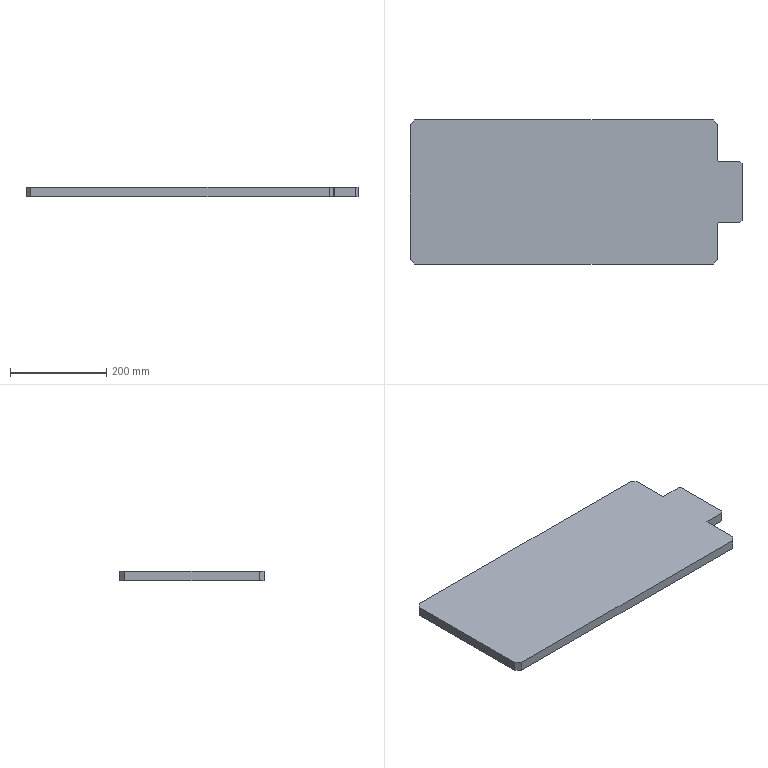Part | SolidWorks | features Chamfer 2, Extrusion 1, Fillet 1 | 1 solid | 18 faces | box 690 x 300 x 20 mm | volume 3963509 mm3 | plane 16 | cylinder 2 | commonest cylinder face diameters 2 x2
STEP:
#1=CARTESIAN_POINT('',(591.229,150.,20.));
#2=VERTEX_POINT('',#1);
#3=CARTESIAN_POINT('',(-28.771,150.,20.));
#4=VERTEX_POINT('',#3);
#5=CARTESIAN_POINT('',(-38.771,150.,20.));
#6=DIRECTION('',(-1.,0.,0.));
#7=VECTOR('',#6,1000.);
#8=LINE('',#5,#7);
#9=EDGE_CURVE('',#2,#4,#8,.T.);
#10=ORIENTED_EDGE('',*,*,#9,.F.);
#11=CARTESIAN_POINT('',(591.229,150.,0.));
#12=VERTEX_POINT('',#11);
#13=CARTESIAN_POINT('',(591.229,150.,20.));
#14=DIRECTION('',(0.,0.,-1.));
#15=VECTOR('',#14,1000.);
#16=LINE('',#13,#15);
#17=EDGE_CURVE('',#2,#12,#16,.T.);
#18=ORIENTED_EDGE('',*,*,#17,.T.);
#19=CARTESIAN_POINT('',(-28.771,150.,0.));
#20=VERTEX_POINT('',#19);
#21=CARTESIAN_POINT('',(-38.771,150.,0.));
#22=DIRECTION('',(-1.,0.,0.));
#23=VECTOR('',#22,1000.);
#24=LINE('',#21,#23);
#25=EDGE_CURVE('',#12,#20,#24,.T.);
#26=ORIENTED_EDGE('',*,*,#25,.T.);
#27=CARTESIAN_POINT('',(-28.771,150.,20.));
#28=DIRECTION('',(0.,0.,1.));
#29=VECTOR('',#28,1000.);
#30=LINE('',#27,#29);
#31=EDGE_CURVE('',#20,#4,#30,.T.);
#32=ORIENTED_EDGE('',*,*,#31,.T.);
#33=EDGE_LOOP('',(#10,#18,#26,#32));
#34=FACE_OUTER_BOUND('',#33,.T.);
#35=CARTESIAN_POINT('',(-38.771,150.,20.));
#36=DIRECTION('',(0.,-1.,0.));
#37=DIRECTION('',(0.,0.,-1.));
#38=AXIS2_PLACEMENT_3D('',#35,#36,#37);
#39=PLANE('',#38);
#40=ADVANCED_FACE('',(#34),#39,.F.);
#41=CARTESIAN_POINT('',(-38.771,140.,0.));
#42=VERTEX_POINT('',#41);
#43=CARTESIAN_POINT('',(-38.771,-140.,0.));
#44=VERTEX_POINT('',#43);
#45=CARTESIAN_POINT('',(-38.771,-150.,0.));
#46=DIRECTION('',(0.,-1.,0.));
#47=VECTOR('',#46,1000.);
#48=LINE('',#45,#47);
#49=EDGE_CURVE('',#42,#44,#48,.T.);
#50=ORIENTED_EDGE('',*,*,#49,.T.);
#51=CARTESIAN_POINT('',(-38.771,-140.,20.));
#52=VERTEX_POINT('',#51);
#53=CARTESIAN_POINT('',(-38.771,-140.,20.));
#54=DIRECTION('',(0.,0.,1.));
#55=VECTOR('',#54,1000.);
#56=LINE('',#53,#55);
#57=EDGE_CURVE('',#44,#52,#56,.T.);
#58=ORIENTED_EDGE('',*,*,#57,.T.);
#59=CARTESIAN_POINT('',(-38.771,140.,20.));
#60=VERTEX_POINT('',#59);
#61=CARTESIAN_POINT('',(-38.771,-150.,20.));
#62=DIRECTION('',(0.,-1.,0.));
#63=VECTOR('',#62,1000.);
#64=LINE('',#61,#63);
#65=EDGE_CURVE('',#60,#52,#64,.T.);
#66=ORIENTED_EDGE('',*,*,#65,.F.);
#67=CARTESIAN_POINT('',(-38.771,140.,20.));
#68=DIRECTION('',(0.,0.,-1.));
#69=VECTOR('',#68,1000.);
#70=LINE('',#67,#69);
#71=EDGE_CURVE('',#60,#42,#70,.T.);
#72=ORIENTED_EDGE('',*,*,#71,.T.);
#73=EDGE_LOOP('',(#50,#58,#66,#72));
#74=FACE_OUTER_BOUND('',#73,.T.);
#75=CARTESIAN_POINT('',(-38.771,-150.,20.));
#76=DIRECTION('',(1.,0.,0.));
#77=DIRECTION('',(0.,0.,-1.));
#78=AXIS2_PLACEMENT_3D('',#75,#76,#77);
#79=PLANE('',#78);
#80=ADVANCED_FACE('',(#74),#79,.F.);
#81=CARTESIAN_POINT('',(-28.771,-150.,0.));
#82=VERTEX_POINT('',#81);
#83=CARTESIAN_POINT('',(591.229,-150.,0.));
#84=VERTEX_POINT('',#83);
#85=CARTESIAN_POINT('',(-38.771,-150.,0.));
#86=DIRECTION('',(1.,0.,0.));
#87=VECTOR('',#86,1000.);
#88=LINE('',#85,#87);
#89=EDGE_CURVE('',#82,#84,#88,.T.);
#90=ORIENTED_EDGE('',*,*,#89,.T.);
#91=CARTESIAN_POINT('',(591.229,-150.,20.));
#92=VERTEX_POINT('',#91);
#93=CARTESIAN_POINT('',(591.229,-150.,20.));
#94=DIRECTION('',(0.,0.,1.));
#95=VECTOR('',#94,1000.);
#96=LINE('',#93,#95);
#97=EDGE_CURVE('',#84,#92,#96,.T.);
#98=ORIENTED_EDGE('',*,*,#97,.T.);
#99=CARTESIAN_POINT('',(-28.771,-150.,20.));
#100=VERTEX_POINT('',#99);
#101=CARTESIAN_POINT('',(-38.771,-150.,20.));
#102=DIRECTION('',(1.,0.,0.));
#103=VECTOR('',#102,1000.);
#104=LINE('',#101,#103);
#105=EDGE_CURVE('',#100,#92,#104,.T.);
#106=ORIENTED_EDGE('',*,*,#105,.F.);
#107=CARTESIAN_POINT('',(-28.771,-150.,20.));
#108=DIRECTION('',(0.,0.,-1.));
#109=VECTOR('',#108,1000.);
#110=LINE('',#107,#109);
#111=EDGE_CURVE('',#100,#82,#110,.T.);
#112=ORIENTED_EDGE('',*,*,#111,.T.);
#113=EDGE_LOOP('',(#90,#98,#106,#112));
#114=FACE_OUTER_BOUND('',#113,.T.);
#115=CARTESIAN_POINT('',(-38.771,-150.,20.));
#116=DIRECTION('',(0.,1.,0.));
#117=DIRECTION('',(0.,0.,1.));
#118=AXIS2_PLACEMENT_3D('',#115,#116,#117);
#119=PLANE('',#118);
#120=ADVANCED_FACE('',(#114),#119,.F.);
#121=CARTESIAN_POINT('',(601.229,-140.,0.));
#122=VERTEX_POINT('',#121);
#123=CARTESIAN_POINT('',(601.229,-65.,0.));
#124=VERTEX_POINT('',#123);
#125=CARTESIAN_POINT('',(601.229,-150.,0.));
#126=DIRECTION('',(0.,1.,0.));
#127=VECTOR('',#126,1000.);
#128=LINE('',#125,#127);
#129=EDGE_CURVE('',#122,#124,#128,.T.);
#130=ORIENTED_EDGE('',*,*,#129,.T.);
#131=CARTESIAN_POINT('',(601.229,-65.,20.));
#132=VERTEX_POINT('',#131);
#133=CARTESIAN_POINT('',(601.229,-65.,20.));
#134=DIRECTION('',(0.,0.,1.));
#135=VECTOR('',#134,1000.);
#136=LINE('',#133,#135);
#137=EDGE_CURVE('',#124,#132,#136,.T.);
#138=ORIENTED_EDGE('',*,*,#137,.T.);
#139=CARTESIAN_POINT('',(601.229,-140.,20.));
#140=VERTEX_POINT('',#139);
#141=CARTESIAN_POINT('',(601.229,-150.,20.));
#142=DIRECTION('',(0.,1.,0.));
#143=VECTOR('',#142,1000.);
#144=LINE('',#141,#143);
#145=EDGE_CURVE('',#140,#132,#144,.T.);
#146=ORIENTED_EDGE('',*,*,#145,.F.);
#147=CARTESIAN_POINT('',(601.229,-140.,20.));
#148=DIRECTION('',(0.,0.,-1.));
#149=VECTOR('',#148,1000.);
#150=LINE('',#147,#149);
#151=EDGE_CURVE('',#140,#122,#150,.T.);
#152=ORIENTED_EDGE('',*,*,#151,.T.);
#153=EDGE_LOOP('',(#130,#138,#146,#152));
#154=FACE_OUTER_BOUND('',#153,.T.);
#155=CARTESIAN_POINT('',(601.229,-150.,20.));
#156=DIRECTION('',(-1.,0.,0.));
#157=DIRECTION('',(0.,0.,1.));
#158=AXIS2_PLACEMENT_3D('',#155,#156,#157);
#159=PLANE('',#158);
#160=ADVANCED_FACE('',(#154),#159,.F.);
#161=CARTESIAN_POINT('',(602.229,-64.,0.));
#162=VERTEX_POINT('',#161);
#163=CARTESIAN_POINT('',(646.229,-64.,0.));
#164=VERTEX_POINT('',#163);
#165=CARTESIAN_POINT('',(601.229,-64.,0.));
#166=DIRECTION('',(1.,0.,0.));
#167=VECTOR('',#166,1000.);
#168=LINE('',#165,#167);
#169=EDGE_CURVE('',#162,#164,#168,.T.);
#170=ORIENTED_EDGE('',*,*,#169,.T.);
#171=CARTESIAN_POINT('',(646.229,-64.,20.));
#172=VERTEX_POINT('',#171);
#173=CARTESIAN_POINT('',(646.229,-64.,20.));
#174=DIRECTION('',(0.,0.,1.));
#175=VECTOR('',#174,1000.);
#176=LINE('',#173,#175);
#177=EDGE_CURVE('',#164,#172,#176,.T.);
#178=ORIENTED_EDGE('',*,*,#177,.T.);
#179=CARTESIAN_POINT('',(602.229,-64.,20.));
#180=VERTEX_POINT('',#179);
#181=CARTESIAN_POINT('',(601.229,-64.,20.));
#182=DIRECTION('',(1.,0.,0.));
#183=VECTOR('',#182,1000.);
#184=LINE('',#181,#183);
#185=EDGE_CURVE('',#180,#172,#184,.T.);
#186=ORIENTED_EDGE('',*,*,#185,.F.);
#187=CARTESIAN_POINT('',(602.229,-64.,0.));
#188=DIRECTION('',(0.,0.,-1.));
#189=VECTOR('',#188,1000.);
#190=LINE('',#187,#189);
#191=EDGE_CURVE('',#180,#162,#190,.T.);
#192=ORIENTED_EDGE('',*,*,#191,.T.);
#193=EDGE_LOOP('',(#170,#178,#186,#192));
#194=FACE_OUTER_BOUND('',#193,.T.);
#195=CARTESIAN_POINT('',(601.229,-64.,20.));
#196=DIRECTION('',(0.,1.,0.));
#197=DIRECTION('',(0.,0.,1.));
#198=AXIS2_PLACEMENT_3D('',#195,#196,#197);
#199=PLANE('',#198);
#200=ADVANCED_FACE('',(#194),#199,.F.);
#201=CARTESIAN_POINT('',(651.229,-59.,20.));
#202=VERTEX_POINT('',#201);
#203=CARTESIAN_POINT('',(651.229,59.,20.));
#204=VERTEX_POINT('',#203);
#205=CARTESIAN_POINT('',(651.229,64.,20.));
#206=DIRECTION('',(0.,1.,0.));
#207=VECTOR('',#206,1000.);
#208=LINE('',#205,#207);
#209=EDGE_CURVE('',#202,#204,#208,.T.);
#210=ORIENTED_EDGE('',*,*,#209,.F.);
#211=CARTESIAN_POINT('',(651.229,-59.,0.));
#212=VERTEX_POINT('',#211);
#213=CARTESIAN_POINT('',(651.229,-59.,20.));
#214=DIRECTION('',(0.,0.,-1.));
#215=VECTOR('',#214,1000.);
#216=LINE('',#213,#215);
#217=EDGE_CURVE('',#202,#212,#216,.T.);
#218=ORIENTED_EDGE('',*,*,#217,.T.);
#219=CARTESIAN_POINT('',(651.229,59.,0.));
#220=VERTEX_POINT('',#219);
#221=CARTESIAN_POINT('',(651.229,64.,0.));
#222=DIRECTION('',(0.,1.,0.));
#223=VECTOR('',#222,1000.);
#224=LINE('',#221,#223);
#225=EDGE_CURVE('',#212,#220,#224,.T.);
#226=ORIENTED_EDGE('',*,*,#225,.T.);
#227=CARTESIAN_POINT('',(651.229,59.,20.));
#228=DIRECTION('',(0.,0.,1.));
#229=VECTOR('',#228,1000.);
#230=LINE('',#227,#229);
#231=EDGE_CURVE('',#220,#204,#230,.T.);
#232=ORIENTED_EDGE('',*,*,#231,.T.);
#233=EDGE_LOOP('',(#210,#218,#226,#232));
#234=FACE_OUTER_BOUND('',#233,.T.);
#235=CARTESIAN_POINT('',(651.229,64.,20.));
#236=DIRECTION('',(-1.,0.,0.));
#237=DIRECTION('',(0.,0.,1.));
#238=AXIS2_PLACEMENT_3D('',#235,#236,#237);
#239=PLANE('',#238);
#240=ADVANCED_FACE('',(#234),#239,.F.);
#241=CARTESIAN_POINT('',(646.229,64.,20.));
#242=VERTEX_POINT('',#241);
#243=CARTESIAN_POINT('',(602.229,64.,20.));
#244=VERTEX_POINT('',#243);
#245=CARTESIAN_POINT('',(601.229,64.,20.));
#246=DIRECTION('',(-1.,0.,0.));
#247=VECTOR('',#246,1000.);
#248=LINE('',#245,#247);
#249=EDGE_CURVE('',#242,#244,#248,.T.);
#250=ORIENTED_EDGE('',*,*,#249,.F.);
#251=CARTESIAN_POINT('',(646.229,64.,0.));
#252=VERTEX_POINT('',#251);
#253=CARTESIAN_POINT('',(646.229,64.,20.));
#254=DIRECTION('',(0.,0.,-1.));
#255=VECTOR('',#254,1000.);
#256=LINE('',#253,#255);
#257=EDGE_CURVE('',#242,#252,#256,.T.);
#258=ORIENTED_EDGE('',*,*,#257,.T.);
#259=CARTESIAN_POINT('',(602.229,64.,0.));
#260=VERTEX_POINT('',#259);
#261=CARTESIAN_POINT('',(601.229,64.,0.));
#262=DIRECTION('',(-1.,0.,0.));
#263=VECTOR('',#262,1000.);
#264=LINE('',#261,#263);
#265=EDGE_CURVE('',#252,#260,#264,.T.);
#266=ORIENTED_EDGE('',*,*,#265,.T.);
#267=CARTESIAN_POINT('',(602.229,64.,20.));
#268=DIRECTION('',(0.,0.,1.));
#269=VECTOR('',#268,1000.);
#270=LINE('',#267,#269);
#271=EDGE_CURVE('',#260,#244,#270,.T.);
#272=ORIENTED_EDGE('',*,*,#271,.T.);
#273=EDGE_LOOP('',(#250,#258,#266,#272));
#274=FACE_OUTER_BOUND('',#273,.T.);
#275=CARTESIAN_POINT('',(601.229,64.,20.));
#276=DIRECTION('',(0.,-1.,0.));
#277=DIRECTION('',(0.,0.,-1.));
#278=AXIS2_PLACEMENT_3D('',#275,#276,#277);
#279=PLANE('',#278);
#280=ADVANCED_FACE('',(#274),#279,.F.);
#281=CARTESIAN_POINT('',(601.229,65.,20.));
#282=VERTEX_POINT('',#281);
#283=CARTESIAN_POINT('',(601.229,140.,20.));
#284=VERTEX_POINT('',#283);
#285=CARTESIAN_POINT('',(601.229,150.,20.));
#286=DIRECTION('',(0.,1.,0.));
#287=VECTOR('',#286,1000.);
#288=LINE('',#285,#287);
#289=EDGE_CURVE('',#282,#284,#288,.T.);
#290=ORIENTED_EDGE('',*,*,#289,.F.);
#291=CARTESIAN_POINT('',(601.229,65.,0.));
#292=VERTEX_POINT('',#291);
#293=CARTESIAN_POINT('',(601.229,65.,0.));
#294=DIRECTION('',(0.,0.,-1.));
#295=VECTOR('',#294,1000.);
#296=LINE('',#293,#295);
#297=EDGE_CURVE('',#282,#292,#296,.T.);
#298=ORIENTED_EDGE('',*,*,#297,.T.);
#299=CARTESIAN_POINT('',(601.229,140.,0.));
#300=VERTEX_POINT('',#299);
#301=CARTESIAN_POINT('',(601.229,150.,0.));
#302=DIRECTION('',(0.,1.,0.));
#303=VECTOR('',#302,1000.);
#304=LINE('',#301,#303);
#305=EDGE_CURVE('',#292,#300,#304,.T.);
#306=ORIENTED_EDGE('',*,*,#305,.T.);
#307=CARTESIAN_POINT('',(601.229,140.,20.));
#308=DIRECTION('',(0.,0.,1.));
#309=VECTOR('',#308,1000.);
#310=LINE('',#307,#309);
#311=EDGE_CURVE('',#300,#284,#310,.T.);
#312=ORIENTED_EDGE('',*,*,#311,.T.);
#313=EDGE_LOOP('',(#290,#298,#306,#312));
#314=FACE_OUTER_BOUND('',#313,.T.);
#315=CARTESIAN_POINT('',(601.229,150.,20.));
#316=DIRECTION('',(-1.,0.,0.));
#317=DIRECTION('',(0.,0.,1.));
#318=AXIS2_PLACEMENT_3D('',#315,#316,#317);
#319=PLANE('',#318);
#320=ADVANCED_FACE('',(#314),#319,.F.);
#321=ORIENTED_EDGE('',*,*,#185,.T.);
#322=CARTESIAN_POINT('',(651.229,-59.,20.));
#323=DIRECTION('',(0.7071,0.7071,0.));
#324=VECTOR('',#323,1000.);
#325=LINE('',#322,#324);
#326=EDGE_CURVE('',#172,#202,#325,.T.);
#327=ORIENTED_EDGE('',*,*,#326,.T.);
#328=ORIENTED_EDGE('',*,*,#209,.T.);
#329=CARTESIAN_POINT('',(646.229,64.,20.));
#330=DIRECTION('',(-0.7071,0.7071,0.));
#331=VECTOR('',#330,1000.);
#332=LINE('',#329,#331);
#333=EDGE_CURVE('',#204,#242,#332,.T.);
#334=ORIENTED_EDGE('',*,*,#333,.T.);
#335=ORIENTED_EDGE('',*,*,#249,.T.);
#336=CARTESIAN_POINT('',(602.229,65.,20.));
#337=DIRECTION('',(0.,0.,-1.));
#338=DIRECTION('',(-1.,0.,0.));
#339=AXIS2_PLACEMENT_3D('',#336,#337,#338);
#340=CIRCLE('',#339,1.);
#341=EDGE_CURVE('',#244,#282,#340,.T.);
#342=ORIENTED_EDGE('',*,*,#341,.T.);
#343=ORIENTED_EDGE('',*,*,#289,.T.);
#344=CARTESIAN_POINT('',(591.229,150.,20.));
#345=DIRECTION('',(-0.7071,0.7071,0.));
#346=VECTOR('',#345,1000.);
#347=LINE('',#344,#346);
#348=EDGE_CURVE('',#284,#2,#347,.T.);
#349=ORIENTED_EDGE('',*,*,#348,.T.);
#350=ORIENTED_EDGE('',*,*,#9,.T.);
#351=CARTESIAN_POINT('',(-38.771,140.,20.));
#352=DIRECTION('',(-0.7071,-0.7071,0.));
#353=VECTOR('',#352,1000.);
#354=LINE('',#351,#353);
#355=EDGE_CURVE('',#4,#60,#354,.T.);
#356=ORIENTED_EDGE('',*,*,#355,.T.);
#357=ORIENTED_EDGE('',*,*,#65,.T.);
#358=CARTESIAN_POINT('',(-28.771,-150.,20.));
#359=DIRECTION('',(0.7071,-0.7071,0.));
#360=VECTOR('',#359,1000.);
#361=LINE('',#358,#360);
#362=EDGE_CURVE('',#52,#100,#361,.T.);
#363=ORIENTED_EDGE('',*,*,#362,.T.);
#364=ORIENTED_EDGE('',*,*,#105,.T.);
#365=CARTESIAN_POINT('',(601.229,-140.,20.));
#366=DIRECTION('',(0.7071,0.7071,0.));
#367=VECTOR('',#366,1000.);
#368=LINE('',#365,#367);
#369=EDGE_CURVE('',#92,#140,#368,.T.);
#370=ORIENTED_EDGE('',*,*,#369,.T.);
#371=ORIENTED_EDGE('',*,*,#145,.T.);
#372=CARTESIAN_POINT('',(602.229,-65.,20.));
#373=DIRECTION('',(0.,0.,-1.));
#374=DIRECTION('',(-1.,0.,0.));
#375=AXIS2_PLACEMENT_3D('',#372,#373,#374);
#376=CIRCLE('',#375,1.);
#377=EDGE_CURVE('',#132,#180,#376,.T.);
#378=ORIENTED_EDGE('',*,*,#377,.T.);
#379=EDGE_LOOP('',(#321,#327,#328,#334,#335,#342,#343,#349,#350,#356,#357,#363,#364,#370,#371,#378));
#380=FACE_OUTER_BOUND('',#379,.T.);
#381=CARTESIAN_POINT('',(0.,0.,20.));
#382=DIRECTION('',(0.,0.,-1.));
#383=DIRECTION('',(-1.,0.,0.));
#384=AXIS2_PLACEMENT_3D('',#381,#382,#383);
#385=PLANE('',#384);
#386=ADVANCED_FACE('',(#380),#385,.F.);
#387=ORIENTED_EDGE('',*,*,#225,.F.);
#388=CARTESIAN_POINT('',(355.115,-355.115,0.));
#389=DIRECTION('',(-0.7071,-0.7071,0.));
#390=VECTOR('',#389,1000.);
#391=LINE('',#388,#390);
#392=EDGE_CURVE('',#212,#164,#391,.T.);
#393=ORIENTED_EDGE('',*,*,#392,.T.);
#394=ORIENTED_EDGE('',*,*,#169,.F.);
#395=CARTESIAN_POINT('',(602.229,-65.,0.));
#396=DIRECTION('',(0.,0.,1.));
#397=DIRECTION('',(-1.,0.,0.));
#398=AXIS2_PLACEMENT_3D('',#395,#396,#397);
#399=CIRCLE('',#398,1.);
#400=EDGE_CURVE('',#162,#124,#399,.T.);
#401=ORIENTED_EDGE('',*,*,#400,.T.);
#402=ORIENTED_EDGE('',*,*,#129,.F.);
#403=CARTESIAN_POINT('',(370.615,-370.615,0.));
#404=DIRECTION('',(-0.7071,-0.7071,0.));
#405=VECTOR('',#404,1000.);
#406=LINE('',#403,#405);
#407=EDGE_CURVE('',#122,#84,#406,.T.);
#408=ORIENTED_EDGE('',*,*,#407,.T.);
#409=ORIENTED_EDGE('',*,*,#89,.F.);
#410=CARTESIAN_POINT('',(-89.385,-89.385,0.));
#411=DIRECTION('',(-0.7071,0.7071,0.));
#412=VECTOR('',#411,1000.);
#413=LINE('',#410,#412);
#414=EDGE_CURVE('',#82,#44,#413,.T.);
#415=ORIENTED_EDGE('',*,*,#414,.T.);
#416=ORIENTED_EDGE('',*,*,#49,.F.);
#417=CARTESIAN_POINT('',(-89.385,89.385,0.));
#418=DIRECTION('',(0.7071,0.7071,0.));
#419=VECTOR('',#418,1000.);
#420=LINE('',#417,#419);
#421=EDGE_CURVE('',#42,#20,#420,.T.);
#422=ORIENTED_EDGE('',*,*,#421,.T.);
#423=ORIENTED_EDGE('',*,*,#25,.F.);
#424=CARTESIAN_POINT('',(370.615,370.615,0.));
#425=DIRECTION('',(0.7071,-0.7071,0.));
#426=VECTOR('',#425,1000.);
#427=LINE('',#424,#426);
#428=EDGE_CURVE('',#12,#300,#427,.T.);
#429=ORIENTED_EDGE('',*,*,#428,.T.);
#430=ORIENTED_EDGE('',*,*,#305,.F.);
#431=CARTESIAN_POINT('',(602.229,65.,0.));
#432=DIRECTION('',(0.,0.,1.));
#433=DIRECTION('',(-1.,0.,0.));
#434=AXIS2_PLACEMENT_3D('',#431,#432,#433);
#435=CIRCLE('',#434,1.);
#436=EDGE_CURVE('',#292,#260,#435,.T.);
#437=ORIENTED_EDGE('',*,*,#436,.T.);
#438=ORIENTED_EDGE('',*,*,#265,.F.);
#439=CARTESIAN_POINT('',(355.115,355.115,0.));
#440=DIRECTION('',(0.7071,-0.7071,0.));
#441=VECTOR('',#440,1000.);
#442=LINE('',#439,#441);
#443=EDGE_CURVE('',#252,#220,#442,.T.);
#444=ORIENTED_EDGE('',*,*,#443,.T.);
#445=EDGE_LOOP('',(#387,#393,#394,#401,#402,#408,#409,#415,#416,#422,#423,#429,#430,#437,#438,#444));
#446=FACE_OUTER_BOUND('',#445,.T.);
#447=CARTESIAN_POINT('',(0.,0.,0.));
#448=DIRECTION('',(0.,0.,-1.));
#449=DIRECTION('',(-1.,0.,0.));
#450=AXIS2_PLACEMENT_3D('',#447,#448,#449);
#451=PLANE('',#450);
#452=ADVANCED_FACE('',(#446),#451,.T.);
#453=ORIENTED_EDGE('',*,*,#348,.F.);
#454=ORIENTED_EDGE('',*,*,#311,.F.);
#455=ORIENTED_EDGE('',*,*,#428,.F.);
#456=ORIENTED_EDGE('',*,*,#17,.F.);
#457=EDGE_LOOP('',(#453,#454,#455,#456));
#458=FACE_OUTER_BOUND('',#457,.T.);
#459=CARTESIAN_POINT('',(591.229,150.,20.));
#460=DIRECTION('',(-0.7071,-0.7071,0.));
#461=DIRECTION('',(0.,0.,-1.));
#462=AXIS2_PLACEMENT_3D('',#459,#460,#461);
#463=PLANE('',#462);
#464=ADVANCED_FACE('',(#458),#463,.F.);
#465=ORIENTED_EDGE('',*,*,#369,.F.);
#466=ORIENTED_EDGE('',*,*,#97,.F.);
#467=ORIENTED_EDGE('',*,*,#407,.F.);
#468=ORIENTED_EDGE('',*,*,#151,.F.);
#469=EDGE_LOOP('',(#465,#466,#467,#468));
#470=FACE_OUTER_BOUND('',#469,.T.);
#471=CARTESIAN_POINT('',(601.229,-140.,20.));
#472=DIRECTION('',(-0.7071,0.7071,0.));
#473=DIRECTION('',(0.,0.,-1.));
#474=AXIS2_PLACEMENT_3D('',#471,#472,#473);
#475=PLANE('',#474);
#476=ADVANCED_FACE('',(#470),#475,.F.);
#477=ORIENTED_EDGE('',*,*,#362,.F.);
#478=ORIENTED_EDGE('',*,*,#57,.F.);
#479=ORIENTED_EDGE('',*,*,#414,.F.);
#480=ORIENTED_EDGE('',*,*,#111,.F.);
#481=EDGE_LOOP('',(#477,#478,#479,#480));
#482=FACE_OUTER_BOUND('',#481,.T.);
#483=CARTESIAN_POINT('',(-28.771,-150.,20.));
#484=DIRECTION('',(0.7071,0.7071,0.));
#485=DIRECTION('',(0.,0.,-1.));
#486=AXIS2_PLACEMENT_3D('',#483,#484,#485);
#487=PLANE('',#486);
#488=ADVANCED_FACE('',(#482),#487,.F.);
#489=ORIENTED_EDGE('',*,*,#355,.F.);
#490=ORIENTED_EDGE('',*,*,#31,.F.);
#491=ORIENTED_EDGE('',*,*,#421,.F.);
#492=ORIENTED_EDGE('',*,*,#71,.F.);
#493=EDGE_LOOP('',(#489,#490,#491,#492));
#494=FACE_OUTER_BOUND('',#493,.T.);
#495=CARTESIAN_POINT('',(-38.771,140.,20.));
#496=DIRECTION('',(0.7071,-0.7071,0.));
#497=DIRECTION('',(0.,0.,-1.));
#498=AXIS2_PLACEMENT_3D('',#495,#496,#497);
#499=PLANE('',#498);
#500=ADVANCED_FACE('',(#494),#499,.F.);
#501=ORIENTED_EDGE('',*,*,#341,.F.);
#502=ORIENTED_EDGE('',*,*,#271,.F.);
#503=ORIENTED_EDGE('',*,*,#436,.F.);
#504=ORIENTED_EDGE('',*,*,#297,.F.);
#505=EDGE_LOOP('',(#501,#502,#503,#504));
#506=FACE_OUTER_BOUND('',#505,.T.);
#507=CARTESIAN_POINT('',(602.229,65.,20.));
#508=DIRECTION('',(0.,0.,1.));
#509=DIRECTION('',(1.,0.,0.));
#510=AXIS2_PLACEMENT_3D('',#507,#508,#509);
#511=CYLINDRICAL_SURFACE('',#510,1.);
#512=ADVANCED_FACE('',(#506),#511,.F.);
#513=ORIENTED_EDGE('',*,*,#377,.F.);
#514=ORIENTED_EDGE('',*,*,#137,.F.);
#515=ORIENTED_EDGE('',*,*,#400,.F.);
#516=ORIENTED_EDGE('',*,*,#191,.F.);
#517=EDGE_LOOP('',(#513,#514,#515,#516));
#518=FACE_OUTER_BOUND('',#517,.T.);
#519=CARTESIAN_POINT('',(602.229,-65.,20.));
#520=DIRECTION('',(0.,0.,1.));
#521=DIRECTION('',(1.,0.,0.));
#522=AXIS2_PLACEMENT_3D('',#519,#520,#521);
#523=CYLINDRICAL_SURFACE('',#522,1.);
#524=ADVANCED_FACE('',(#518),#523,.F.);
#525=ORIENTED_EDGE('',*,*,#326,.F.);
#526=ORIENTED_EDGE('',*,*,#177,.F.);
#527=ORIENTED_EDGE('',*,*,#392,.F.);
#528=ORIENTED_EDGE('',*,*,#217,.F.);
#529=EDGE_LOOP('',(#525,#526,#527,#528));
#530=FACE_OUTER_BOUND('',#529,.T.);
#531=CARTESIAN_POINT('',(651.229,-59.,20.));
#532=DIRECTION('',(-0.7071,0.7071,0.));
#533=DIRECTION('',(0.,0.,-1.));
#534=AXIS2_PLACEMENT_3D('',#531,#532,#533);
#535=PLANE('',#534);
#536=ADVANCED_FACE('',(#530),#535,.F.);
#537=ORIENTED_EDGE('',*,*,#333,.F.);
#538=ORIENTED_EDGE('',*,*,#231,.F.);
#539=ORIENTED_EDGE('',*,*,#443,.F.);
#540=ORIENTED_EDGE('',*,*,#257,.F.);
#541=EDGE_LOOP('',(#537,#538,#539,#540));
#542=FACE_OUTER_BOUND('',#541,.T.);
#543=CARTESIAN_POINT('',(646.229,64.,20.));
#544=DIRECTION('',(-0.7071,-0.7071,0.));
#545=DIRECTION('',(0.,0.,-1.));
#546=AXIS2_PLACEMENT_3D('',#543,#544,#545);
#547=PLANE('',#546);
#548=ADVANCED_FACE('',(#542),#547,.F.);
#549=CLOSED_SHELL('',(#40,#80,#120,#160,#200,#240,#280,#320,#386,#452,#464,#476,#488,#500,#512,#524,#536,#548));
#550=MANIFOLD_SOLID_BREP('',#549);
#551=CARTESIAN_POINT('',(0.,0.,0.));
#552=DIRECTION('',(0.,0.,1.));
#553=DIRECTION('',(1.,0.,0.));
#554=AXIS2_PLACEMENT_3D('',#551,#552,#553);
#555=(LENGTH_UNIT()NAMED_UNIT(*)SI_UNIT(.MILLI.,.METRE.));
#556=UNCERTAINTY_MEASURE_WITH_UNIT(LENGTH_MEASURE(0.00001),#555,'','');
#557=(NAMED_UNIT(*)PLANE_ANGLE_UNIT()SI_UNIT($,.RADIAN.));
#558=(NAMED_UNIT(*)SI_UNIT($,.STERADIAN.)SOLID_ANGLE_UNIT());
#559=(GEOMETRIC_REPRESENTATION_CONTEXT(3)GLOBAL_UNCERTAINTY_ASSIGNED_CONTEXT((#556))GLOBAL_UNIT_ASSIGNED_CONTEXT((#555,#557,#558))REPRESENTATION_CONTEXT('',''));
#560=ADVANCED_BREP_SHAPE_REPRESENTATION('',(#550,#554),#559);